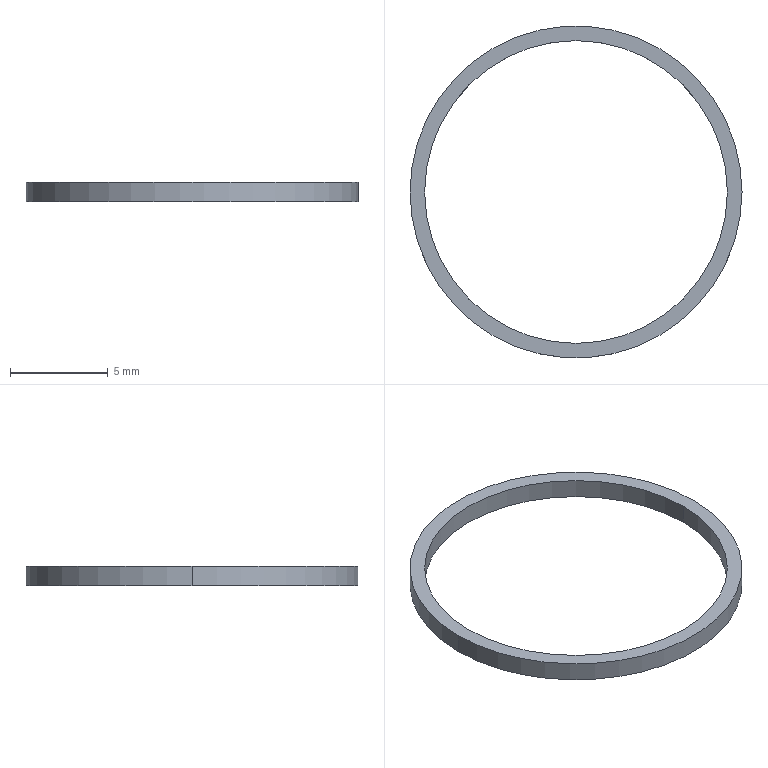Part | STEP file | Extension spring | 1 solid | 6 faces | box 17 x 17 x 1 mm | volume 38.288 mm3 | cylinder 4 | plane 2 | commonest cylinder face diameters 15.5 x2 17 x2
STEP:
#1=CARTESIAN_POINT('',(0.,0.,0.));
#2=DIRECTION('',(0.,0.,1.));
#3=DIRECTION('',(1.,0.,0.));
#4=AXIS2_PLACEMENT_3D('',#1,#2,#3);
#5=CARTESIAN_POINT('',(-7.75,0.,1.));
#6=VERTEX_POINT('',#5);
#7=CARTESIAN_POINT('',(-7.75,0.,0.));
#8=VERTEX_POINT('',#7);
#9=CARTESIAN_POINT('',(-7.75,0.,1.));
#10=DIRECTION('',(0.,0.,-1.));
#11=VECTOR('',#10,1.);
#12=LINE('',#9,#11);
#13=CARTESIAN_POINT('',(0.,0.,1.));
#14=DIRECTION('',(0.,0.,-1.));
#15=DIRECTION('',(-1.,0.,0.));
#16=AXIS2_PLACEMENT_3D('',#13,#14,#15);
#17=CYLINDRICAL_SURFACE('',#16,7.75);
#18=CARTESIAN_POINT('',(6.283,0.));
#19=DIRECTION('',(0.,1.));
#20=VECTOR('',#19,1.);
#21=LINE('',#18,#20);
#22=(GEOMETRIC_REPRESENTATION_CONTEXT(2)PARAMETRIC_REPRESENTATION_CONTEXT()REPRESENTATION_CONTEXT('',''));
#23=DEFINITIONAL_REPRESENTATION('',(#21),#22);
#24=PCURVE('',#17,#23);
#25=CARTESIAN_POINT('',(0.,0.,1.));
#26=DIRECTION('',(0.,0.,-1.));
#27=DIRECTION('',(-1.,0.,0.));
#28=AXIS2_PLACEMENT_3D('',#25,#26,#27);
#29=CYLINDRICAL_SURFACE('',#28,7.75);
#30=CARTESIAN_POINT('',(0.,0.));
#31=DIRECTION('',(0.,1.));
#32=VECTOR('',#31,1.);
#33=LINE('',#30,#32);
#34=(GEOMETRIC_REPRESENTATION_CONTEXT(2)PARAMETRIC_REPRESENTATION_CONTEXT()REPRESENTATION_CONTEXT('',''));
#35=DEFINITIONAL_REPRESENTATION('',(#33),#34);
#36=PCURVE('',#29,#35);
#37=SURFACE_CURVE('',#12,(#24,#36),.PCURVE_S1.);
#38=EDGE_CURVE('',#6,#8,#37,.T.);
#39=ORIENTED_EDGE('',*,*,#38,.T.);
#40=CARTESIAN_POINT('',(7.75,0.,0.));
#41=VERTEX_POINT('',#40);
#42=CARTESIAN_POINT('',(0.,0.,0.));
#43=DIRECTION('',(0.,0.,1.));
#44=DIRECTION('',(-1.,0.,0.));
#45=AXIS2_PLACEMENT_3D('',#42,#43,#44);
#46=CIRCLE('',#45,7.75);
#47=CARTESIAN_POINT('',(6.283,1.));
#48=DIRECTION('',(-1.,0.));
#49=VECTOR('',#48,1.);
#50=LINE('',#47,#49);
#51=(GEOMETRIC_REPRESENTATION_CONTEXT(2)PARAMETRIC_REPRESENTATION_CONTEXT()REPRESENTATION_CONTEXT('',''));
#52=DEFINITIONAL_REPRESENTATION('',(#50),#51);
#53=PCURVE('',#17,#52);
#54=CARTESIAN_POINT('',(0.,0.,0.));
#55=DIRECTION('',(0.,0.,1.));
#56=DIRECTION('',(1.,0.,0.));
#57=AXIS2_PLACEMENT_3D('',#54,#55,#56);
#58=PLANE('',#57);
#59=CARTESIAN_POINT('',(0.,0.));
#60=DIRECTION('',(-1.,0.));
#61=AXIS2_PLACEMENT_2D('',#59,#60);
#62=CIRCLE('',#61,7.75);
#63=(GEOMETRIC_REPRESENTATION_CONTEXT(2)PARAMETRIC_REPRESENTATION_CONTEXT()REPRESENTATION_CONTEXT('',''));
#64=DEFINITIONAL_REPRESENTATION('',(#62),#63);
#65=PCURVE('',#58,#64);
#66=SURFACE_CURVE('',#46,(#53,#65),.PCURVE_S1.);
#67=EDGE_CURVE('',#8,#41,#66,.T.);
#68=ORIENTED_EDGE('',*,*,#67,.T.);
#69=CARTESIAN_POINT('',(7.75,0.,1.));
#70=VERTEX_POINT('',#69);
#71=CARTESIAN_POINT('',(7.75,0.,1.));
#72=DIRECTION('',(0.,0.,-1.));
#73=VECTOR('',#72,1.);
#74=LINE('',#71,#73);
#75=CARTESIAN_POINT('',(3.142,0.));
#76=DIRECTION('',(0.,1.));
#77=VECTOR('',#76,1.);
#78=LINE('',#75,#77);
#79=(GEOMETRIC_REPRESENTATION_CONTEXT(2)PARAMETRIC_REPRESENTATION_CONTEXT()REPRESENTATION_CONTEXT('',''));
#80=DEFINITIONAL_REPRESENTATION('',(#78),#79);
#81=PCURVE('',#17,#80);
#82=CARTESIAN_POINT('',(3.142,0.));
#83=DIRECTION('',(0.,1.));
#84=VECTOR('',#83,1.);
#85=LINE('',#82,#84);
#86=(GEOMETRIC_REPRESENTATION_CONTEXT(2)PARAMETRIC_REPRESENTATION_CONTEXT()REPRESENTATION_CONTEXT('',''));
#87=DEFINITIONAL_REPRESENTATION('',(#85),#86);
#88=PCURVE('',#29,#87);
#89=SURFACE_CURVE('',#74,(#81,#88),.PCURVE_S1.);
#90=EDGE_CURVE('',#70,#41,#89,.T.);
#91=ORIENTED_EDGE('',*,*,#90,.F.);
#92=CARTESIAN_POINT('',(0.,0.,1.));
#93=DIRECTION('',(0.,0.,-1.));
#94=DIRECTION('',(-1.,0.,0.));
#95=AXIS2_PLACEMENT_3D('',#92,#93,#94);
#96=CIRCLE('',#95,7.75);
#97=CARTESIAN_POINT('',(0.,0.));
#98=DIRECTION('',(1.,0.));
#99=VECTOR('',#98,1.);
#100=LINE('',#97,#99);
#101=(GEOMETRIC_REPRESENTATION_CONTEXT(2)PARAMETRIC_REPRESENTATION_CONTEXT()REPRESENTATION_CONTEXT('',''));
#102=DEFINITIONAL_REPRESENTATION('',(#100),#101);
#103=PCURVE('',#17,#102);
#104=CARTESIAN_POINT('',(0.,0.,1.));
#105=DIRECTION('',(0.,0.,1.));
#106=DIRECTION('',(1.,0.,0.));
#107=AXIS2_PLACEMENT_3D('',#104,#105,#106);
#108=PLANE('',#107);
#109=CARTESIAN_POINT('',(-7.75,0.));
#110=CARTESIAN_POINT('',(-7.75,13.423));
#111=CARTESIAN_POINT('',(3.875,6.712));
#112=CARTESIAN_POINT('',(15.5,0.));
#113=CARTESIAN_POINT('',(3.875,-6.712));
#114=CARTESIAN_POINT('',(-7.75,-13.423));
#115=CARTESIAN_POINT('',(-7.75,0.));
#116=(BOUNDED_CURVE()B_SPLINE_CURVE(2,(#109,#110,#111,#112,#113,#114,#115),.UNSPECIFIED.,.T.,.F.)B_SPLINE_CURVE_WITH_KNOTS((1,2,2,2,2,1),(-2.094,0.,2.094,4.189,6.283,8.378),.UNSPECIFIED.)CURVE()GEOMETRIC_REPRESENTATION_ITEM()RATIONAL_B_SPLINE_CURVE((1.,0.5,1.,0.5,1.,0.5,1.))REPRESENTATION_ITEM(''));
#117=(GEOMETRIC_REPRESENTATION_CONTEXT(2)PARAMETRIC_REPRESENTATION_CONTEXT()REPRESENTATION_CONTEXT('',''));
#118=DEFINITIONAL_REPRESENTATION('',(#116),#117);
#119=PCURVE('',#108,#118);
#120=SURFACE_CURVE('',#96,(#103,#119),.PCURVE_S1.);
#121=EDGE_CURVE('',#70,#6,#120,.T.);
#122=ORIENTED_EDGE('',*,*,#121,.T.);
#123=EDGE_LOOP('',(#39,#68,#91,#122));
#124=FACE_BOUND('',#123,.F.);
#125=ADVANCED_FACE('',(#124),#17,.F.);
#126=CARTESIAN_POINT('',(8.5,0.,1.));
#127=VERTEX_POINT('',#126);
#128=CARTESIAN_POINT('',(-8.5,0.,1.));
#129=VERTEX_POINT('',#128);
#130=CARTESIAN_POINT('',(0.,0.,1.));
#131=DIRECTION('',(0.,0.,1.));
#132=DIRECTION('',(-1.,0.,0.));
#133=AXIS2_PLACEMENT_3D('',#130,#131,#132);
#134=CIRCLE('',#133,8.5);
#135=CARTESIAN_POINT('',(0.,0.,1.));
#136=DIRECTION('',(0.,0.,-1.));
#137=DIRECTION('',(-1.,0.,0.));
#138=AXIS2_PLACEMENT_3D('',#135,#136,#137);
#139=CYLINDRICAL_SURFACE('',#138,8.5);
#140=CARTESIAN_POINT('',(6.283,0.));
#141=DIRECTION('',(-1.,0.));
#142=VECTOR('',#141,1.);
#143=LINE('',#140,#142);
#144=(GEOMETRIC_REPRESENTATION_CONTEXT(2)PARAMETRIC_REPRESENTATION_CONTEXT()REPRESENTATION_CONTEXT('',''));
#145=DEFINITIONAL_REPRESENTATION('',(#143),#144);
#146=PCURVE('',#139,#145);
#147=CARTESIAN_POINT('',(0.,0.));
#148=DIRECTION('',(-1.,0.));
#149=AXIS2_PLACEMENT_2D('',#147,#148);
#150=CIRCLE('',#149,8.5);
#151=(GEOMETRIC_REPRESENTATION_CONTEXT(2)PARAMETRIC_REPRESENTATION_CONTEXT()REPRESENTATION_CONTEXT('',''));
#152=DEFINITIONAL_REPRESENTATION('',(#150),#151);
#153=PCURVE('',#108,#152);
#154=SURFACE_CURVE('',#134,(#146,#153),.PCURVE_S1.);
#155=EDGE_CURVE('',#127,#129,#154,.T.);
#156=ORIENTED_EDGE('',*,*,#155,.F.);
#157=CARTESIAN_POINT('',(8.5,0.,0.));
#158=VERTEX_POINT('',#157);
#159=CARTESIAN_POINT('',(8.5,0.,1.));
#160=DIRECTION('',(0.,0.,-1.));
#161=VECTOR('',#160,1.);
#162=LINE('',#159,#161);
#163=CARTESIAN_POINT('',(3.142,0.));
#164=DIRECTION('',(0.,1.));
#165=VECTOR('',#164,1.);
#166=LINE('',#163,#165);
#167=(GEOMETRIC_REPRESENTATION_CONTEXT(2)PARAMETRIC_REPRESENTATION_CONTEXT()REPRESENTATION_CONTEXT('',''));
#168=DEFINITIONAL_REPRESENTATION('',(#166),#167);
#169=PCURVE('',#139,#168);
#170=CARTESIAN_POINT('',(0.,0.,1.));
#171=DIRECTION('',(0.,0.,-1.));
#172=DIRECTION('',(-1.,0.,0.));
#173=AXIS2_PLACEMENT_3D('',#170,#171,#172);
#174=CYLINDRICAL_SURFACE('',#173,8.5);
#175=CARTESIAN_POINT('',(3.142,0.));
#176=DIRECTION('',(0.,1.));
#177=VECTOR('',#176,1.);
#178=LINE('',#175,#177);
#179=(GEOMETRIC_REPRESENTATION_CONTEXT(2)PARAMETRIC_REPRESENTATION_CONTEXT()REPRESENTATION_CONTEXT('',''));
#180=DEFINITIONAL_REPRESENTATION('',(#178),#179);
#181=PCURVE('',#174,#180);
#182=SURFACE_CURVE('',#162,(#169,#181),.PCURVE_S1.);
#183=EDGE_CURVE('',#127,#158,#182,.T.);
#184=ORIENTED_EDGE('',*,*,#183,.T.);
#185=CARTESIAN_POINT('',(-8.5,0.,0.));
#186=VERTEX_POINT('',#185);
#187=CARTESIAN_POINT('',(0.,0.,0.));
#188=DIRECTION('',(0.,0.,1.));
#189=DIRECTION('',(-1.,0.,0.));
#190=AXIS2_PLACEMENT_3D('',#187,#188,#189);
#191=CIRCLE('',#190,8.5);
#192=CARTESIAN_POINT('',(6.283,1.));
#193=DIRECTION('',(-1.,0.));
#194=VECTOR('',#193,1.);
#195=LINE('',#192,#194);
#196=(GEOMETRIC_REPRESENTATION_CONTEXT(2)PARAMETRIC_REPRESENTATION_CONTEXT()REPRESENTATION_CONTEXT('',''));
#197=DEFINITIONAL_REPRESENTATION('',(#195),#196);
#198=PCURVE('',#139,#197);
#199=CARTESIAN_POINT('',(0.,0.));
#200=DIRECTION('',(-1.,0.));
#201=AXIS2_PLACEMENT_2D('',#199,#200);
#202=CIRCLE('',#201,8.5);
#203=(GEOMETRIC_REPRESENTATION_CONTEXT(2)PARAMETRIC_REPRESENTATION_CONTEXT()REPRESENTATION_CONTEXT('',''));
#204=DEFINITIONAL_REPRESENTATION('',(#202),#203);
#205=PCURVE('',#58,#204);
#206=SURFACE_CURVE('',#191,(#198,#205),.PCURVE_S1.);
#207=EDGE_CURVE('',#158,#186,#206,.T.);
#208=ORIENTED_EDGE('',*,*,#207,.T.);
#209=CARTESIAN_POINT('',(-8.5,0.,1.));
#210=DIRECTION('',(0.,0.,-1.));
#211=VECTOR('',#210,1.);
#212=LINE('',#209,#211);
#213=CARTESIAN_POINT('',(0.,0.));
#214=DIRECTION('',(0.,1.));
#215=VECTOR('',#214,1.);
#216=LINE('',#213,#215);
#217=(GEOMETRIC_REPRESENTATION_CONTEXT(2)PARAMETRIC_REPRESENTATION_CONTEXT()REPRESENTATION_CONTEXT('',''));
#218=DEFINITIONAL_REPRESENTATION('',(#216),#217);
#219=PCURVE('',#139,#218);
#220=CARTESIAN_POINT('',(6.283,0.));
#221=DIRECTION('',(0.,1.));
#222=VECTOR('',#221,1.);
#223=LINE('',#220,#222);
#224=(GEOMETRIC_REPRESENTATION_CONTEXT(2)PARAMETRIC_REPRESENTATION_CONTEXT()REPRESENTATION_CONTEXT('',''));
#225=DEFINITIONAL_REPRESENTATION('',(#223),#224);
#226=PCURVE('',#174,#225);
#227=SURFACE_CURVE('',#212,(#219,#226),.PCURVE_S1.);
#228=EDGE_CURVE('',#129,#186,#227,.T.);
#229=ORIENTED_EDGE('',*,*,#228,.F.);
#230=EDGE_LOOP('',(#156,#184,#208,#229));
#231=FACE_BOUND('',#230,.T.);
#232=ADVANCED_FACE('',(#231),#139,.T.);
#233=CARTESIAN_POINT('',(0.,0.,1.));
#234=DIRECTION('',(0.,0.,-1.));
#235=DIRECTION('',(-1.,0.,0.));
#236=AXIS2_PLACEMENT_3D('',#233,#234,#235);
#237=CIRCLE('',#236,7.75);
#238=CARTESIAN_POINT('',(-7.75,0.));
#239=CARTESIAN_POINT('',(-7.75,13.423));
#240=CARTESIAN_POINT('',(3.875,6.712));
#241=CARTESIAN_POINT('',(15.5,0.));
#242=CARTESIAN_POINT('',(3.875,-6.712));
#243=CARTESIAN_POINT('',(-7.75,-13.423));
#244=CARTESIAN_POINT('',(-7.75,0.));
#245=(BOUNDED_CURVE()B_SPLINE_CURVE(2,(#238,#239,#240,#241,#242,#243,#244),.UNSPECIFIED.,.T.,.F.)B_SPLINE_CURVE_WITH_KNOTS((1,2,2,2,2,1),(-2.094,0.,2.094,4.189,6.283,8.378),.UNSPECIFIED.)CURVE()GEOMETRIC_REPRESENTATION_ITEM()RATIONAL_B_SPLINE_CURVE((1.,0.5,1.,0.5,1.,0.5,1.))REPRESENTATION_ITEM(''));
#246=(GEOMETRIC_REPRESENTATION_CONTEXT(2)PARAMETRIC_REPRESENTATION_CONTEXT()REPRESENTATION_CONTEXT('',''));
#247=DEFINITIONAL_REPRESENTATION('',(#245),#246);
#248=PCURVE('',#108,#247);
#249=CARTESIAN_POINT('',(0.,0.));
#250=DIRECTION('',(1.,0.));
#251=VECTOR('',#250,1.);
#252=LINE('',#249,#251);
#253=(GEOMETRIC_REPRESENTATION_CONTEXT(2)PARAMETRIC_REPRESENTATION_CONTEXT()REPRESENTATION_CONTEXT('',''));
#254=DEFINITIONAL_REPRESENTATION('',(#252),#253);
#255=PCURVE('',#29,#254);
#256=SURFACE_CURVE('',#237,(#248,#255),.PCURVE_S1.);
#257=EDGE_CURVE('',#6,#70,#256,.T.);
#258=ORIENTED_EDGE('',*,*,#257,.T.);
#259=ORIENTED_EDGE('',*,*,#121,.T.);
#260=EDGE_LOOP('',(#258,#259));
#261=FACE_BOUND('',#260,.T.);
#262=CARTESIAN_POINT('',(0.,0.,1.));
#263=DIRECTION('',(0.,0.,1.));
#264=DIRECTION('',(-1.,0.,0.));
#265=AXIS2_PLACEMENT_3D('',#262,#263,#264);
#266=CIRCLE('',#265,8.5);
#267=CARTESIAN_POINT('',(0.,0.));
#268=DIRECTION('',(-1.,0.));
#269=AXIS2_PLACEMENT_2D('',#267,#268);
#270=CIRCLE('',#269,8.5);
#271=(GEOMETRIC_REPRESENTATION_CONTEXT(2)PARAMETRIC_REPRESENTATION_CONTEXT()REPRESENTATION_CONTEXT('',''));
#272=DEFINITIONAL_REPRESENTATION('',(#270),#271);
#273=PCURVE('',#108,#272);
#274=CARTESIAN_POINT('',(6.283,0.));
#275=DIRECTION('',(-1.,0.));
#276=VECTOR('',#275,1.);
#277=LINE('',#274,#276);
#278=(GEOMETRIC_REPRESENTATION_CONTEXT(2)PARAMETRIC_REPRESENTATION_CONTEXT()REPRESENTATION_CONTEXT('',''));
#279=DEFINITIONAL_REPRESENTATION('',(#277),#278);
#280=PCURVE('',#174,#279);
#281=SURFACE_CURVE('',#266,(#273,#280),.PCURVE_S1.);
#282=EDGE_CURVE('',#129,#127,#281,.T.);
#283=ORIENTED_EDGE('',*,*,#282,.T.);
#284=ORIENTED_EDGE('',*,*,#155,.T.);
#285=EDGE_LOOP('',(#283,#284));
#286=FACE_BOUND('',#285,.T.);
#287=ADVANCED_FACE('',(#261,#286),#108,.T.);
#288=CARTESIAN_POINT('',(0.,0.,0.));
#289=DIRECTION('',(0.,0.,1.));
#290=DIRECTION('',(-1.,0.,0.));
#291=AXIS2_PLACEMENT_3D('',#288,#289,#290);
#292=CIRCLE('',#291,7.75);
#293=CARTESIAN_POINT('',(6.283,1.));
#294=DIRECTION('',(-1.,0.));
#295=VECTOR('',#294,1.);
#296=LINE('',#293,#295);
#297=(GEOMETRIC_REPRESENTATION_CONTEXT(2)PARAMETRIC_REPRESENTATION_CONTEXT()REPRESENTATION_CONTEXT('',''));
#298=DEFINITIONAL_REPRESENTATION('',(#296),#297);
#299=PCURVE('',#29,#298);
#300=CARTESIAN_POINT('',(0.,0.));
#301=DIRECTION('',(-1.,0.));
#302=AXIS2_PLACEMENT_2D('',#300,#301);
#303=CIRCLE('',#302,7.75);
#304=(GEOMETRIC_REPRESENTATION_CONTEXT(2)PARAMETRIC_REPRESENTATION_CONTEXT()REPRESENTATION_CONTEXT('',''));
#305=DEFINITIONAL_REPRESENTATION('',(#303),#304);
#306=PCURVE('',#58,#305);
#307=SURFACE_CURVE('',#292,(#299,#306),.PCURVE_S1.);
#308=EDGE_CURVE('',#41,#8,#307,.T.);
#309=ORIENTED_EDGE('',*,*,#308,.T.);
#310=ORIENTED_EDGE('',*,*,#38,.F.);
#311=ORIENTED_EDGE('',*,*,#257,.T.);
#312=ORIENTED_EDGE('',*,*,#90,.T.);
#313=EDGE_LOOP('',(#309,#310,#311,#312));
#314=FACE_BOUND('',#313,.F.);
#315=ADVANCED_FACE('',(#314),#29,.F.);
#316=ORIENTED_EDGE('',*,*,#183,.F.);
#317=ORIENTED_EDGE('',*,*,#282,.F.);
#318=ORIENTED_EDGE('',*,*,#228,.T.);
#319=CARTESIAN_POINT('',(0.,0.,0.));
#320=DIRECTION('',(0.,0.,1.));
#321=DIRECTION('',(-1.,0.,0.));
#322=AXIS2_PLACEMENT_3D('',#319,#320,#321);
#323=CIRCLE('',#322,8.5);
#324=CARTESIAN_POINT('',(6.283,1.));
#325=DIRECTION('',(-1.,0.));
#326=VECTOR('',#325,1.);
#327=LINE('',#324,#326);
#328=(GEOMETRIC_REPRESENTATION_CONTEXT(2)PARAMETRIC_REPRESENTATION_CONTEXT()REPRESENTATION_CONTEXT('',''));
#329=DEFINITIONAL_REPRESENTATION('',(#327),#328);
#330=PCURVE('',#174,#329);
#331=CARTESIAN_POINT('',(0.,0.));
#332=DIRECTION('',(-1.,0.));
#333=AXIS2_PLACEMENT_2D('',#331,#332);
#334=CIRCLE('',#333,8.5);
#335=(GEOMETRIC_REPRESENTATION_CONTEXT(2)PARAMETRIC_REPRESENTATION_CONTEXT()REPRESENTATION_CONTEXT('',''));
#336=DEFINITIONAL_REPRESENTATION('',(#334),#335);
#337=PCURVE('',#58,#336);
#338=SURFACE_CURVE('',#323,(#330,#337),.PCURVE_S1.);
#339=EDGE_CURVE('',#186,#158,#338,.T.);
#340=ORIENTED_EDGE('',*,*,#339,.T.);
#341=EDGE_LOOP('',(#316,#317,#318,#340));
#342=FACE_BOUND('',#341,.T.);
#343=ADVANCED_FACE('',(#342),#174,.T.);
#344=ORIENTED_EDGE('',*,*,#67,.T.);
#345=ORIENTED_EDGE('',*,*,#308,.T.);
#346=EDGE_LOOP('',(#344,#345));
#347=FACE_BOUND('',#346,.T.);
#348=ORIENTED_EDGE('',*,*,#339,.F.);
#349=ORIENTED_EDGE('',*,*,#207,.F.);
#350=EDGE_LOOP('',(#348,#349));
#351=FACE_BOUND('',#350,.T.);
#352=ADVANCED_FACE('',(#347,#351),#58,.F.);
#353=CLOSED_SHELL('',(#125,#232,#287,#315,#343,#352));
#354=MANIFOLD_SOLID_BREP('',#353);
#355=(LENGTH_UNIT()NAMED_UNIT(*)SI_UNIT(.MILLI.,.METRE.));
#356=UNCERTAINTY_MEASURE_WITH_UNIT(LENGTH_MEASURE(0.0000001),#355,'','');
#357=(NAMED_UNIT(*)PLANE_ANGLE_UNIT()SI_UNIT($,.RADIAN.));
#358=(NAMED_UNIT(*)SI_UNIT($,.STERADIAN.)SOLID_ANGLE_UNIT());
#359=(GEOMETRIC_REPRESENTATION_CONTEXT(3)GLOBAL_UNCERTAINTY_ASSIGNED_CONTEXT((#356))GLOBAL_UNIT_ASSIGNED_CONTEXT((#355,#357,#358))REPRESENTATION_CONTEXT('',''));
#360=ADVANCED_BREP_SHAPE_REPRESENTATION('',(#4,#354),#359);